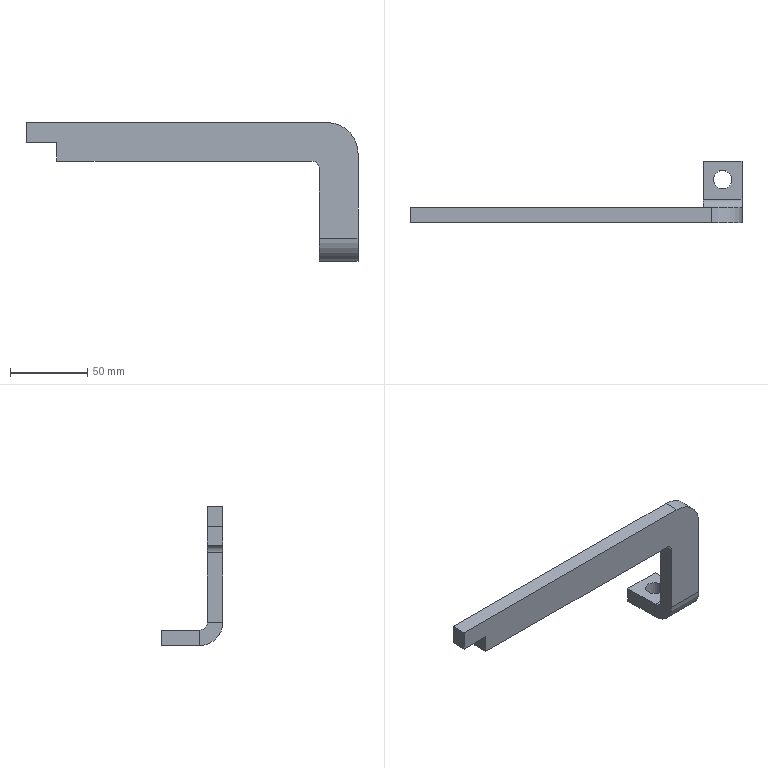Part | STEP file | Produce dryer HY-40-M-702 | 1 solid | 22 faces | box 215 x 40 x 90 mm | volume 72091 mm3 | plane 16 | cylinder 6 | commonest cylinder face diameters 10 x2 12 x2 30 x1 40 x1
STEP:
#1=CARTESIAN_POINT('',(196.5,18.,-90.));
#2=VERTEX_POINT('',#1);
#3=CARTESIAN_POINT('',(208.5,18.,-90.));
#4=VERTEX_POINT('',#3);
#5=CARTESIAN_POINT('',(202.5,18.,-90.));
#6=DIRECTION('',(0.,0.,1.));
#7=DIRECTION('',(1.,0.,0.));
#8=AXIS2_PLACEMENT_3D('',#5,#6,#7);
#9=CIRCLE('',#8,6.);
#10=EDGE_CURVE('',#2,#4,#9,.T.);
#11=ORIENTED_EDGE('',*,*,#10,.F.);
#12=CARTESIAN_POINT('',(196.5,18.,-80.));
#13=VERTEX_POINT('',#12);
#14=CARTESIAN_POINT('',(196.5,18.,-90.));
#15=DIRECTION('',(0.,0.,1.));
#16=VECTOR('',#15,1000.);
#17=LINE('',#14,#16);
#18=EDGE_CURVE('',#2,#13,#17,.T.);
#19=ORIENTED_EDGE('',*,*,#18,.T.);
#20=CARTESIAN_POINT('',(208.5,18.,-80.));
#21=VERTEX_POINT('',#20);
#22=CARTESIAN_POINT('',(202.5,18.,-80.));
#23=DIRECTION('',(0.,0.,1.));
#24=DIRECTION('',(1.,0.,0.));
#25=AXIS2_PLACEMENT_3D('',#22,#23,#24);
#26=CIRCLE('',#25,6.);
#27=EDGE_CURVE('',#13,#21,#26,.T.);
#28=ORIENTED_EDGE('',*,*,#27,.T.);
#29=CARTESIAN_POINT('',(208.5,18.,-90.));
#30=DIRECTION('',(0.,0.,1.));
#31=VECTOR('',#30,1000.);
#32=LINE('',#29,#31);
#33=EDGE_CURVE('',#4,#21,#32,.T.);
#34=ORIENTED_EDGE('',*,*,#33,.F.);
#35=EDGE_LOOP('',(#11,#19,#28,#34));
#36=FACE_OUTER_BOUND('',#35,.T.);
#37=CARTESIAN_POINT('',(202.5,18.,-90.));
#38=DIRECTION('',(0.,0.,1.));
#39=DIRECTION('',(1.,0.,0.));
#40=AXIS2_PLACEMENT_3D('',#37,#38,#39);
#41=CYLINDRICAL_SURFACE('',#40,6.);
#42=ADVANCED_FACE('',(#36),#41,.F.);
#43=CARTESIAN_POINT('',(190.,0.,-75.));
#44=VERTEX_POINT('',#43);
#45=CARTESIAN_POINT('',(190.,0.,-30.));
#46=VERTEX_POINT('',#45);
#47=CARTESIAN_POINT('',(190.,0.,-90.));
#48=DIRECTION('',(0.,0.,1.));
#49=VECTOR('',#48,1000.);
#50=LINE('',#47,#49);
#51=EDGE_CURVE('',#44,#46,#50,.T.);
#52=ORIENTED_EDGE('',*,*,#51,.F.);
#53=CARTESIAN_POINT('',(190.,-10.,-75.));
#54=VERTEX_POINT('',#53);
#55=CARTESIAN_POINT('',(190.,0.,-75.));
#56=DIRECTION('',(0.,-1.,0.));
#57=VECTOR('',#56,1000.);
#58=LINE('',#55,#57);
#59=EDGE_CURVE('',#44,#54,#58,.T.);
#60=ORIENTED_EDGE('',*,*,#59,.T.);
#61=CARTESIAN_POINT('',(190.,-10.,-30.));
#62=VERTEX_POINT('',#61);
#63=CARTESIAN_POINT('',(190.,-10.,-90.));
#64=DIRECTION('',(0.,0.,1.));
#65=VECTOR('',#64,1000.);
#66=LINE('',#63,#65);
#67=EDGE_CURVE('',#54,#62,#66,.T.);
#68=ORIENTED_EDGE('',*,*,#67,.T.);
#69=CARTESIAN_POINT('',(190.,-10.,-30.));
#70=DIRECTION('',(0.,1.,0.));
#71=VECTOR('',#70,1000.);
#72=LINE('',#69,#71);
#73=EDGE_CURVE('',#62,#46,#72,.T.);
#74=ORIENTED_EDGE('',*,*,#73,.T.);
#75=EDGE_LOOP('',(#52,#60,#68,#74));
#76=FACE_OUTER_BOUND('',#75,.T.);
#77=CARTESIAN_POINT('',(190.,-10.,-90.));
#78=DIRECTION('',(-1.,0.,0.));
#79=DIRECTION('',(0.,0.,1.));
#80=AXIS2_PLACEMENT_3D('',#77,#78,#79);
#81=PLANE('',#80);
#82=ADVANCED_FACE('',(#76),#81,.T.);
#83=CARTESIAN_POINT('',(215.,-10.,-75.));
#84=VERTEX_POINT('',#83);
#85=CARTESIAN_POINT('',(190.,-10.,-75.));
#86=DIRECTION('',(1.,0.,0.));
#87=VECTOR('',#86,1000.);
#88=LINE('',#85,#87);
#89=EDGE_CURVE('',#54,#84,#88,.T.);
#90=ORIENTED_EDGE('',*,*,#89,.T.);
#91=CARTESIAN_POINT('',(215.,-10.,-20.));
#92=VERTEX_POINT('',#91);
#93=CARTESIAN_POINT('',(215.,-10.,-20.));
#94=DIRECTION('',(0.,0.,-1.));
#95=VECTOR('',#94,1000.);
#96=LINE('',#93,#95);
#97=EDGE_CURVE('',#92,#84,#96,.T.);
#98=ORIENTED_EDGE('',*,*,#97,.F.);
#99=CARTESIAN_POINT('',(195.,-10.,0.));
#100=VERTEX_POINT('',#99);
#101=CARTESIAN_POINT('',(195.,-10.,-20.));
#102=DIRECTION('',(0.,1.,0.));
#103=DIRECTION('',(0.,0.,1.));
#104=AXIS2_PLACEMENT_3D('',#101,#102,#103);
#105=CIRCLE('',#104,20.);
#106=EDGE_CURVE('',#100,#92,#105,.T.);
#107=ORIENTED_EDGE('',*,*,#106,.F.);
#108=CARTESIAN_POINT('',(0.,-10.,0.));
#109=VERTEX_POINT('',#108);
#110=CARTESIAN_POINT('',(0.,-10.,0.));
#111=DIRECTION('',(1.,0.,0.));
#112=VECTOR('',#111,1000.);
#113=LINE('',#110,#112);
#114=EDGE_CURVE('',#109,#100,#113,.T.);
#115=ORIENTED_EDGE('',*,*,#114,.F.);
#116=CARTESIAN_POINT('',(0.,-10.,-13.));
#117=VERTEX_POINT('',#116);
#118=CARTESIAN_POINT('',(0.,-10.,-13.));
#119=DIRECTION('',(0.,0.,1.));
#120=VECTOR('',#119,1000.);
#121=LINE('',#118,#120);
#122=EDGE_CURVE('',#117,#109,#121,.T.);
#123=ORIENTED_EDGE('',*,*,#122,.F.);
#124=CARTESIAN_POINT('',(20.,-10.,-13.));
#125=VERTEX_POINT('',#124);
#126=CARTESIAN_POINT('',(0.,-10.,-13.));
#127=DIRECTION('',(-1.,0.,0.));
#128=VECTOR('',#127,1000.);
#129=LINE('',#126,#128);
#130=EDGE_CURVE('',#125,#117,#129,.T.);
#131=ORIENTED_EDGE('',*,*,#130,.F.);
#132=CARTESIAN_POINT('',(20.,-10.,-25.));
#133=VERTEX_POINT('',#132);
#134=CARTESIAN_POINT('',(20.,-10.,-25.));
#135=DIRECTION('',(0.,0.,1.));
#136=VECTOR('',#135,1000.);
#137=LINE('',#134,#136);
#138=EDGE_CURVE('',#133,#125,#137,.T.);
#139=ORIENTED_EDGE('',*,*,#138,.F.);
#140=CARTESIAN_POINT('',(185.,-10.,-25.));
#141=VERTEX_POINT('',#140);
#142=CARTESIAN_POINT('',(185.,-10.,-25.));
#143=DIRECTION('',(-1.,0.,0.));
#144=VECTOR('',#143,1000.);
#145=LINE('',#142,#144);
#146=EDGE_CURVE('',#141,#133,#145,.T.);
#147=ORIENTED_EDGE('',*,*,#146,.F.);
#148=CARTESIAN_POINT('',(185.,-10.,-30.));
#149=DIRECTION('',(0.,-1.,0.));
#150=DIRECTION('',(0.,0.,-1.));
#151=AXIS2_PLACEMENT_3D('',#148,#149,#150);
#152=CIRCLE('',#151,5.);
#153=EDGE_CURVE('',#62,#141,#152,.T.);
#154=ORIENTED_EDGE('',*,*,#153,.F.);
#155=ORIENTED_EDGE('',*,*,#67,.F.);
#156=EDGE_LOOP('',(#90,#98,#107,#115,#123,#131,#139,#147,#154,#155));
#157=FACE_OUTER_BOUND('',#156,.T.);
#158=CARTESIAN_POINT('',(195.,-10.,-20.));
#159=DIRECTION('',(0.,1.,0.));
#160=DIRECTION('',(0.,0.,1.));
#161=AXIS2_PLACEMENT_3D('',#158,#159,#160);
#162=PLANE('',#161);
#163=ADVANCED_FACE('',(#157),#162,.F.);
#164=CARTESIAN_POINT('',(215.,0.,-20.));
#165=VERTEX_POINT('',#164);
#166=CARTESIAN_POINT('',(215.,0.,-75.));
#167=VERTEX_POINT('',#166);
#168=CARTESIAN_POINT('',(215.,0.,-20.));
#169=DIRECTION('',(0.,0.,-1.));
#170=VECTOR('',#169,1000.);
#171=LINE('',#168,#170);
#172=EDGE_CURVE('',#165,#167,#171,.T.);
#173=ORIENTED_EDGE('',*,*,#172,.T.);
#174=CARTESIAN_POINT('',(190.,0.,-75.));
#175=DIRECTION('',(1.,0.,0.));
#176=VECTOR('',#175,1000.);
#177=LINE('',#174,#176);
#178=EDGE_CURVE('',#44,#167,#177,.T.);
#179=ORIENTED_EDGE('',*,*,#178,.F.);
#180=ORIENTED_EDGE('',*,*,#51,.T.);
#181=CARTESIAN_POINT('',(185.,0.,-25.));
#182=VERTEX_POINT('',#181);
#183=CARTESIAN_POINT('',(185.,0.,-30.));
#184=DIRECTION('',(0.,-1.,0.));
#185=DIRECTION('',(0.,0.,-1.));
#186=AXIS2_PLACEMENT_3D('',#183,#184,#185);
#187=CIRCLE('',#186,5.);
#188=EDGE_CURVE('',#46,#182,#187,.T.);
#189=ORIENTED_EDGE('',*,*,#188,.T.);
#190=CARTESIAN_POINT('',(20.,0.,-25.));
#191=VERTEX_POINT('',#190);
#192=CARTESIAN_POINT('',(185.,0.,-25.));
#193=DIRECTION('',(-1.,0.,0.));
#194=VECTOR('',#193,1000.);
#195=LINE('',#192,#194);
#196=EDGE_CURVE('',#182,#191,#195,.T.);
#197=ORIENTED_EDGE('',*,*,#196,.T.);
#198=CARTESIAN_POINT('',(20.,0.,-13.));
#199=VERTEX_POINT('',#198);
#200=CARTESIAN_POINT('',(20.,0.,-25.));
#201=DIRECTION('',(0.,0.,1.));
#202=VECTOR('',#201,1000.);
#203=LINE('',#200,#202);
#204=EDGE_CURVE('',#191,#199,#203,.T.);
#205=ORIENTED_EDGE('',*,*,#204,.T.);
#206=CARTESIAN_POINT('',(0.,0.,-13.));
#207=VERTEX_POINT('',#206);
#208=CARTESIAN_POINT('',(0.,0.,-13.));
#209=DIRECTION('',(-1.,0.,0.));
#210=VECTOR('',#209,1000.);
#211=LINE('',#208,#210);
#212=EDGE_CURVE('',#199,#207,#211,.T.);
#213=ORIENTED_EDGE('',*,*,#212,.T.);
#214=CARTESIAN_POINT('',(0.,0.,0.));
#215=VERTEX_POINT('',#214);
#216=CARTESIAN_POINT('',(0.,0.,-13.));
#217=DIRECTION('',(0.,0.,1.));
#218=VECTOR('',#217,1000.);
#219=LINE('',#216,#218);
#220=EDGE_CURVE('',#207,#215,#219,.T.);
#221=ORIENTED_EDGE('',*,*,#220,.T.);
#222=CARTESIAN_POINT('',(195.,0.,0.));
#223=VERTEX_POINT('',#222);
#224=CARTESIAN_POINT('',(0.,0.,0.));
#225=DIRECTION('',(1.,0.,0.));
#226=VECTOR('',#225,1000.);
#227=LINE('',#224,#226);
#228=EDGE_CURVE('',#215,#223,#227,.T.);
#229=ORIENTED_EDGE('',*,*,#228,.T.);
#230=CARTESIAN_POINT('',(195.,0.,-20.));
#231=DIRECTION('',(0.,1.,0.));
#232=DIRECTION('',(0.,0.,1.));
#233=AXIS2_PLACEMENT_3D('',#230,#231,#232);
#234=CIRCLE('',#233,20.);
#235=EDGE_CURVE('',#223,#165,#234,.T.);
#236=ORIENTED_EDGE('',*,*,#235,.T.);
#237=EDGE_LOOP('',(#173,#179,#180,#189,#197,#205,#213,#221,#229,#236));
#238=FACE_OUTER_BOUND('',#237,.T.);
#239=CARTESIAN_POINT('',(195.,0.,-20.));
#240=DIRECTION('',(0.,1.,0.));
#241=DIRECTION('',(0.,0.,1.));
#242=AXIS2_PLACEMENT_3D('',#239,#240,#241);
#243=PLANE('',#242);
#244=ADVANCED_FACE('',(#238),#243,.T.);
#245=ORIENTED_EDGE('',*,*,#220,.F.);
#246=CARTESIAN_POINT('',(0.,-10.,-13.));
#247=DIRECTION('',(0.,1.,0.));
#248=VECTOR('',#247,1000.);
#249=LINE('',#246,#248);
#250=EDGE_CURVE('',#117,#207,#249,.T.);
#251=ORIENTED_EDGE('',*,*,#250,.F.);
#252=ORIENTED_EDGE('',*,*,#122,.T.);
#253=CARTESIAN_POINT('',(0.,-10.,0.));
#254=DIRECTION('',(0.,1.,0.));
#255=VECTOR('',#254,1000.);
#256=LINE('',#253,#255);
#257=EDGE_CURVE('',#109,#215,#256,.T.);
#258=ORIENTED_EDGE('',*,*,#257,.T.);
#259=EDGE_LOOP('',(#245,#251,#252,#258));
#260=FACE_OUTER_BOUND('',#259,.T.);
#261=CARTESIAN_POINT('',(0.,-10.,-13.));
#262=DIRECTION('',(-1.,0.,0.));
#263=DIRECTION('',(0.,0.,1.));
#264=AXIS2_PLACEMENT_3D('',#261,#262,#263);
#265=PLANE('',#264);
#266=ADVANCED_FACE('',(#260),#265,.T.);
#267=ORIENTED_EDGE('',*,*,#212,.F.);
#268=CARTESIAN_POINT('',(20.,-10.,-13.));
#269=DIRECTION('',(0.,1.,0.));
#270=VECTOR('',#269,1000.);
#271=LINE('',#268,#270);
#272=EDGE_CURVE('',#125,#199,#271,.T.);
#273=ORIENTED_EDGE('',*,*,#272,.F.);
#274=ORIENTED_EDGE('',*,*,#130,.T.);
#275=ORIENTED_EDGE('',*,*,#250,.T.);
#276=EDGE_LOOP('',(#267,#273,#274,#275));
#277=FACE_OUTER_BOUND('',#276,.T.);
#278=CARTESIAN_POINT('',(0.,-10.,-13.));
#279=DIRECTION('',(0.,0.,-1.));
#280=DIRECTION('',(-1.,0.,0.));
#281=AXIS2_PLACEMENT_3D('',#278,#279,#280);
#282=PLANE('',#281);
#283=ADVANCED_FACE('',(#277),#282,.T.);
#284=ORIENTED_EDGE('',*,*,#204,.F.);
#285=CARTESIAN_POINT('',(20.,-10.,-25.));
#286=DIRECTION('',(0.,1.,0.));
#287=VECTOR('',#286,1000.);
#288=LINE('',#285,#287);
#289=EDGE_CURVE('',#133,#191,#288,.T.);
#290=ORIENTED_EDGE('',*,*,#289,.F.);
#291=ORIENTED_EDGE('',*,*,#138,.T.);
#292=ORIENTED_EDGE('',*,*,#272,.T.);
#293=EDGE_LOOP('',(#284,#290,#291,#292));
#294=FACE_OUTER_BOUND('',#293,.T.);
#295=CARTESIAN_POINT('',(20.,-10.,-25.));
#296=DIRECTION('',(-1.,0.,0.));
#297=DIRECTION('',(0.,0.,1.));
#298=AXIS2_PLACEMENT_3D('',#295,#296,#297);
#299=PLANE('',#298);
#300=ADVANCED_FACE('',(#294),#299,.T.);
#301=ORIENTED_EDGE('',*,*,#196,.F.);
#302=CARTESIAN_POINT('',(185.,-10.,-25.));
#303=DIRECTION('',(0.,1.,0.));
#304=VECTOR('',#303,1000.);
#305=LINE('',#302,#304);
#306=EDGE_CURVE('',#141,#182,#305,.T.);
#307=ORIENTED_EDGE('',*,*,#306,.F.);
#308=ORIENTED_EDGE('',*,*,#146,.T.);
#309=ORIENTED_EDGE('',*,*,#289,.T.);
#310=EDGE_LOOP('',(#301,#307,#308,#309));
#311=FACE_OUTER_BOUND('',#310,.T.);
#312=CARTESIAN_POINT('',(185.,-10.,-25.));
#313=DIRECTION('',(0.,0.,-1.));
#314=DIRECTION('',(-1.,0.,0.));
#315=AXIS2_PLACEMENT_3D('',#312,#313,#314);
#316=PLANE('',#315);
#317=ADVANCED_FACE('',(#311),#316,.T.);
#318=ORIENTED_EDGE('',*,*,#188,.F.);
#319=ORIENTED_EDGE('',*,*,#73,.F.);
#320=ORIENTED_EDGE('',*,*,#153,.T.);
#321=ORIENTED_EDGE('',*,*,#306,.T.);
#322=EDGE_LOOP('',(#318,#319,#320,#321));
#323=FACE_OUTER_BOUND('',#322,.T.);
#324=CARTESIAN_POINT('',(185.,-10.,-30.));
#325=DIRECTION('',(0.,1.,0.));
#326=DIRECTION('',(0.,0.,1.));
#327=AXIS2_PLACEMENT_3D('',#324,#325,#326);
#328=CYLINDRICAL_SURFACE('',#327,5.);
#329=ADVANCED_FACE('',(#323),#328,.F.);
#330=CARTESIAN_POINT('',(215.,0.,-75.));
#331=DIRECTION('',(0.,-1.,0.));
#332=VECTOR('',#331,1000.);
#333=LINE('',#330,#332);
#334=EDGE_CURVE('',#167,#84,#333,.T.);
#335=ORIENTED_EDGE('',*,*,#334,.F.);
#336=ORIENTED_EDGE('',*,*,#172,.F.);
#337=CARTESIAN_POINT('',(215.,-10.,-20.));
#338=DIRECTION('',(0.,1.,0.));
#339=VECTOR('',#338,1000.);
#340=LINE('',#337,#339);
#341=EDGE_CURVE('',#92,#165,#340,.T.);
#342=ORIENTED_EDGE('',*,*,#341,.F.);
#343=ORIENTED_EDGE('',*,*,#97,.T.);
#344=EDGE_LOOP('',(#335,#336,#342,#343));
#345=FACE_OUTER_BOUND('',#344,.T.);
#346=CARTESIAN_POINT('',(215.,-10.,-20.));
#347=DIRECTION('',(1.,0.,0.));
#348=DIRECTION('',(0.,0.,-1.));
#349=AXIS2_PLACEMENT_3D('',#346,#347,#348);
#350=PLANE('',#349);
#351=ADVANCED_FACE('',(#345),#350,.T.);
#352=ORIENTED_EDGE('',*,*,#235,.F.);
#353=CARTESIAN_POINT('',(195.,-10.,0.));
#354=DIRECTION('',(0.,1.,0.));
#355=VECTOR('',#354,1000.);
#356=LINE('',#353,#355);
#357=EDGE_CURVE('',#100,#223,#356,.T.);
#358=ORIENTED_EDGE('',*,*,#357,.F.);
#359=ORIENTED_EDGE('',*,*,#106,.T.);
#360=ORIENTED_EDGE('',*,*,#341,.T.);
#361=EDGE_LOOP('',(#352,#358,#359,#360));
#362=FACE_OUTER_BOUND('',#361,.T.);
#363=CARTESIAN_POINT('',(195.,-10.,-20.));
#364=DIRECTION('',(0.,1.,0.));
#365=DIRECTION('',(0.,0.,1.));
#366=AXIS2_PLACEMENT_3D('',#363,#364,#365);
#367=CYLINDRICAL_SURFACE('',#366,20.);
#368=ADVANCED_FACE('',(#362),#367,.T.);
#369=ORIENTED_EDGE('',*,*,#228,.F.);
#370=ORIENTED_EDGE('',*,*,#257,.F.);
#371=ORIENTED_EDGE('',*,*,#114,.T.);
#372=ORIENTED_EDGE('',*,*,#357,.T.);
#373=EDGE_LOOP('',(#369,#370,#371,#372));
#374=FACE_OUTER_BOUND('',#373,.T.);
#375=CARTESIAN_POINT('',(0.,-10.,0.));
#376=DIRECTION('',(0.,0.,1.));
#377=DIRECTION('',(1.,0.,0.));
#378=AXIS2_PLACEMENT_3D('',#375,#376,#377);
#379=PLANE('',#378);
#380=ADVANCED_FACE('',(#374),#379,.T.);
#381=CARTESIAN_POINT('',(215.,5.,-80.));
#382=VERTEX_POINT('',#381);
#383=CARTESIAN_POINT('',(215.,5.,-90.));
#384=VERTEX_POINT('',#383);
#385=CARTESIAN_POINT('',(215.,5.,-90.));
#386=DIRECTION('',(0.,0.,-1.));
#387=VECTOR('',#386,1000.);
#388=LINE('',#385,#387);
#389=EDGE_CURVE('',#382,#384,#388,.T.);
#390=ORIENTED_EDGE('',*,*,#389,.F.);
#391=CARTESIAN_POINT('',(215.,5.,-75.));
#392=DIRECTION('',(1.,0.,0.));
#393=DIRECTION('',(0.,0.,1.));
#394=AXIS2_PLACEMENT_3D('',#391,#392,#393);
#395=CIRCLE('',#394,5.);
#396=EDGE_CURVE('',#167,#382,#395,.T.);
#397=ORIENTED_EDGE('',*,*,#396,.F.);
#398=ORIENTED_EDGE('',*,*,#334,.T.);
#399=CARTESIAN_POINT('',(215.,5.,-75.));
#400=DIRECTION('',(1.,0.,0.));
#401=DIRECTION('',(0.,0.,1.));
#402=AXIS2_PLACEMENT_3D('',#399,#400,#401);
#403=CIRCLE('',#402,15.);
#404=EDGE_CURVE('',#84,#384,#403,.T.);
#405=ORIENTED_EDGE('',*,*,#404,.T.);
#406=EDGE_LOOP('',(#390,#397,#398,#405));
#407=FACE_OUTER_BOUND('',#406,.T.);
#408=CARTESIAN_POINT('',(215.,5.,-75.));
#409=DIRECTION('',(1.,0.,0.));
#410=DIRECTION('',(0.,0.,-1.));
#411=AXIS2_PLACEMENT_3D('',#408,#409,#410);
#412=PLANE('',#411);
#413=ADVANCED_FACE('',(#407),#412,.T.);
#414=CARTESIAN_POINT('',(190.,5.,-80.));
#415=VERTEX_POINT('',#414);
#416=CARTESIAN_POINT('',(190.,5.,-75.));
#417=DIRECTION('',(-1.,0.,0.));
#418=DIRECTION('',(0.,0.,1.));
#419=AXIS2_PLACEMENT_3D('',#416,#417,#418);
#420=CIRCLE('',#419,5.);
#421=EDGE_CURVE('',#415,#44,#420,.T.);
#422=ORIENTED_EDGE('',*,*,#421,.F.);
#423=CARTESIAN_POINT('',(190.,5.,-90.));
#424=VERTEX_POINT('',#423);
#425=CARTESIAN_POINT('',(190.,5.,-80.));
#426=DIRECTION('',(0.,0.,-1.));
#427=VECTOR('',#426,1000.);
#428=LINE('',#425,#427);
#429=EDGE_CURVE('',#415,#424,#428,.T.);
#430=ORIENTED_EDGE('',*,*,#429,.T.);
#431=CARTESIAN_POINT('',(190.,5.,-75.));
#432=DIRECTION('',(-1.,0.,0.));
#433=DIRECTION('',(0.,0.,1.));
#434=AXIS2_PLACEMENT_3D('',#431,#432,#433);
#435=CIRCLE('',#434,15.);
#436=EDGE_CURVE('',#424,#54,#435,.T.);
#437=ORIENTED_EDGE('',*,*,#436,.T.);
#438=ORIENTED_EDGE('',*,*,#59,.F.);
#439=EDGE_LOOP('',(#422,#430,#437,#438));
#440=FACE_OUTER_BOUND('',#439,.T.);
#441=CARTESIAN_POINT('',(190.,5.,-75.));
#442=DIRECTION('',(1.,0.,0.));
#443=DIRECTION('',(0.,0.,-1.));
#444=AXIS2_PLACEMENT_3D('',#441,#442,#443);
#445=PLANE('',#444);
#446=ADVANCED_FACE('',(#440),#445,.F.);
#447=ORIENTED_EDGE('',*,*,#89,.F.);
#448=ORIENTED_EDGE('',*,*,#436,.F.);
#449=CARTESIAN_POINT('',(0.,5.,-90.));
#450=DIRECTION('',(-1.,0.,0.));
#451=VECTOR('',#450,1000.);
#452=LINE('',#449,#451);
#453=EDGE_CURVE('',#384,#424,#452,.T.);
#454=ORIENTED_EDGE('',*,*,#453,.F.);
#455=ORIENTED_EDGE('',*,*,#404,.F.);
#456=EDGE_LOOP('',(#447,#448,#454,#455));
#457=FACE_OUTER_BOUND('',#456,.T.);
#458=CARTESIAN_POINT('',(190.,5.,-75.));
#459=DIRECTION('',(-1.,0.,0.));
#460=DIRECTION('',(0.,0.,-1.));
#461=AXIS2_PLACEMENT_3D('',#458,#459,#460);
#462=CYLINDRICAL_SURFACE('',#461,15.);
#463=ADVANCED_FACE('',(#457),#462,.T.);
#464=ORIENTED_EDGE('',*,*,#178,.T.);
#465=ORIENTED_EDGE('',*,*,#396,.T.);
#466=CARTESIAN_POINT('',(215.,5.,-80.));
#467=DIRECTION('',(-1.,0.,0.));
#468=VECTOR('',#467,1000.);
#469=LINE('',#466,#468);
#470=EDGE_CURVE('',#382,#415,#469,.T.);
#471=ORIENTED_EDGE('',*,*,#470,.T.);
#472=ORIENTED_EDGE('',*,*,#421,.T.);
#473=EDGE_LOOP('',(#464,#465,#471,#472));
#474=FACE_OUTER_BOUND('',#473,.T.);
#475=CARTESIAN_POINT('',(190.,5.,-75.));
#476=DIRECTION('',(-1.,0.,0.));
#477=DIRECTION('',(0.,0.,-1.));
#478=AXIS2_PLACEMENT_3D('',#475,#476,#477);
#479=CYLINDRICAL_SURFACE('',#478,5.);
#480=ADVANCED_FACE('',(#474),#479,.F.);
#481=CARTESIAN_POINT('',(190.,30.,-90.));
#482=VERTEX_POINT('',#481);
#483=CARTESIAN_POINT('',(190.,0.,-90.));
#484=DIRECTION('',(0.,-1.,0.));
#485=VECTOR('',#484,1000.);
#486=LINE('',#483,#485);
#487=EDGE_CURVE('',#482,#424,#486,.T.);
#488=ORIENTED_EDGE('',*,*,#487,.T.);
#489=ORIENTED_EDGE('',*,*,#429,.F.);
#490=CARTESIAN_POINT('',(190.,30.,-80.));
#491=VERTEX_POINT('',#490);
#492=CARTESIAN_POINT('',(190.,0.,-80.));
#493=DIRECTION('',(0.,-1.,0.));
#494=VECTOR('',#493,1000.);
#495=LINE('',#492,#494);
#496=EDGE_CURVE('',#491,#415,#495,.T.);
#497=ORIENTED_EDGE('',*,*,#496,.F.);
#498=CARTESIAN_POINT('',(190.,30.,-90.));
#499=DIRECTION('',(0.,0.,1.));
#500=VECTOR('',#499,1000.);
#501=LINE('',#498,#500);
#502=EDGE_CURVE('',#482,#491,#501,.T.);
#503=ORIENTED_EDGE('',*,*,#502,.F.);
#504=EDGE_LOOP('',(#488,#489,#497,#503));
#505=FACE_OUTER_BOUND('',#504,.T.);
#506=CARTESIAN_POINT('',(190.,0.,-90.));
#507=DIRECTION('',(-1.,0.,0.));
#508=DIRECTION('',(0.,0.,1.));
#509=AXIS2_PLACEMENT_3D('',#506,#507,#508);
#510=PLANE('',#509);
#511=ADVANCED_FACE('',(#505),#510,.T.);
#512=CARTESIAN_POINT('',(215.,30.,-80.));
#513=VERTEX_POINT('',#512);
#514=CARTESIAN_POINT('',(215.,0.,-80.));
#515=DIRECTION('',(0.,1.,0.));
#516=VECTOR('',#515,1000.);
#517=LINE('',#514,#516);
#518=EDGE_CURVE('',#382,#513,#517,.T.);
#519=ORIENTED_EDGE('',*,*,#518,.F.);
#520=ORIENTED_EDGE('',*,*,#389,.T.);
#521=CARTESIAN_POINT('',(215.,30.,-90.));
#522=VERTEX_POINT('',#521);
#523=CARTESIAN_POINT('',(215.,30.,-90.));
#524=DIRECTION('',(0.,1.,0.));
#525=VECTOR('',#524,1000.);
#526=LINE('',#523,#525);
#527=EDGE_CURVE('',#384,#522,#526,.T.);
#528=ORIENTED_EDGE('',*,*,#527,.T.);
#529=CARTESIAN_POINT('',(215.,30.,-90.));
#530=DIRECTION('',(0.,0.,1.));
#531=VECTOR('',#530,1000.);
#532=LINE('',#529,#531);
#533=EDGE_CURVE('',#522,#513,#532,.T.);
#534=ORIENTED_EDGE('',*,*,#533,.T.);
#535=EDGE_LOOP('',(#519,#520,#528,#534));
#536=FACE_OUTER_BOUND('',#535,.T.);
#537=CARTESIAN_POINT('',(215.,30.,-90.));
#538=DIRECTION('',(1.,0.,0.));
#539=DIRECTION('',(0.,0.,-1.));
#540=AXIS2_PLACEMENT_3D('',#537,#538,#539);
#541=PLANE('',#540);
#542=ADVANCED_FACE('',(#536),#541,.T.);
#543=CARTESIAN_POINT('',(202.5,18.,-90.));
#544=DIRECTION('',(0.,0.,1.));
#545=DIRECTION('',(1.,0.,0.));
#546=AXIS2_PLACEMENT_3D('',#543,#544,#545);
#547=CIRCLE('',#546,6.);
#548=EDGE_CURVE('',#4,#2,#547,.T.);
#549=ORIENTED_EDGE('',*,*,#548,.T.);
#550=ORIENTED_EDGE('',*,*,#10,.T.);
#551=EDGE_LOOP('',(#549,#550));
#552=FACE_BOUND('',#551,.T.);
#553=ORIENTED_EDGE('',*,*,#527,.F.);
#554=ORIENTED_EDGE('',*,*,#453,.T.);
#555=ORIENTED_EDGE('',*,*,#487,.F.);
#556=CARTESIAN_POINT('',(190.,30.,-90.));
#557=DIRECTION('',(-1.,0.,0.));
#558=VECTOR('',#557,1000.);
#559=LINE('',#556,#558);
#560=EDGE_CURVE('',#522,#482,#559,.T.);
#561=ORIENTED_EDGE('',*,*,#560,.F.);
#562=EDGE_LOOP('',(#553,#554,#555,#561));
#563=FACE_OUTER_BOUND('',#562,.T.);
#564=CARTESIAN_POINT('',(0.,0.,-90.));
#565=DIRECTION('',(0.,0.,-1.));
#566=DIRECTION('',(-1.,0.,0.));
#567=AXIS2_PLACEMENT_3D('',#564,#565,#566);
#568=PLANE('',#567);
#569=ADVANCED_FACE('',(#552,#563),#568,.T.);
#570=CARTESIAN_POINT('',(202.5,18.,-80.));
#571=DIRECTION('',(0.,0.,1.));
#572=DIRECTION('',(1.,0.,0.));
#573=AXIS2_PLACEMENT_3D('',#570,#571,#572);
#574=CIRCLE('',#573,6.);
#575=EDGE_CURVE('',#21,#13,#574,.T.);
#576=ORIENTED_EDGE('',*,*,#575,.F.);
#577=ORIENTED_EDGE('',*,*,#27,.F.);
#578=EDGE_LOOP('',(#576,#577));
#579=FACE_BOUND('',#578,.T.);
#580=ORIENTED_EDGE('',*,*,#470,.F.);
#581=ORIENTED_EDGE('',*,*,#518,.T.);
#582=CARTESIAN_POINT('',(0.,30.,-80.));
#583=DIRECTION('',(-1.,0.,0.));
#584=VECTOR('',#583,1000.);
#585=LINE('',#582,#584);
#586=EDGE_CURVE('',#513,#491,#585,.T.);
#587=ORIENTED_EDGE('',*,*,#586,.T.);
#588=ORIENTED_EDGE('',*,*,#496,.T.);
#589=EDGE_LOOP('',(#580,#581,#587,#588));
#590=FACE_OUTER_BOUND('',#589,.T.);
#591=CARTESIAN_POINT('',(0.,0.,-80.));
#592=DIRECTION('',(0.,0.,-1.));
#593=DIRECTION('',(-1.,0.,0.));
#594=AXIS2_PLACEMENT_3D('',#591,#592,#593);
#595=PLANE('',#594);
#596=ADVANCED_FACE('',(#579,#590),#595,.F.);
#597=ORIENTED_EDGE('',*,*,#586,.F.);
#598=ORIENTED_EDGE('',*,*,#533,.F.);
#599=ORIENTED_EDGE('',*,*,#560,.T.);
#600=ORIENTED_EDGE('',*,*,#502,.T.);
#601=EDGE_LOOP('',(#597,#598,#599,#600));
#602=FACE_OUTER_BOUND('',#601,.T.);
#603=CARTESIAN_POINT('',(190.,30.,-90.));
#604=DIRECTION('',(0.,1.,0.));
#605=DIRECTION('',(0.,0.,1.));
#606=AXIS2_PLACEMENT_3D('',#603,#604,#605);
#607=PLANE('',#606);
#608=ADVANCED_FACE('',(#602),#607,.T.);
#609=ORIENTED_EDGE('',*,*,#18,.F.);
#610=ORIENTED_EDGE('',*,*,#548,.F.);
#611=ORIENTED_EDGE('',*,*,#33,.T.);
#612=ORIENTED_EDGE('',*,*,#575,.T.);
#613=EDGE_LOOP('',(#609,#610,#611,#612));
#614=FACE_OUTER_BOUND('',#613,.T.);
#615=CARTESIAN_POINT('',(202.5,18.,-90.));
#616=DIRECTION('',(0.,0.,1.));
#617=DIRECTION('',(1.,0.,0.));
#618=AXIS2_PLACEMENT_3D('',#615,#616,#617);
#619=CYLINDRICAL_SURFACE('',#618,6.);
#620=ADVANCED_FACE('',(#614),#619,.F.);
#621=CLOSED_SHELL('',(#42,#82,#163,#244,#266,#283,#300,#317,#329,#351,#368,#380,#413,#446,#463,#480,#511,#542,#569,#596,#608,#620));
#622=MANIFOLD_SOLID_BREP('',#621);
#623=CARTESIAN_POINT('',(0.,0.,0.));
#624=DIRECTION('',(0.,0.,1.));
#625=DIRECTION('',(1.,0.,0.));
#626=AXIS2_PLACEMENT_3D('',#623,#624,#625);
#627=(LENGTH_UNIT()NAMED_UNIT(*)SI_UNIT(.MILLI.,.METRE.));
#628=UNCERTAINTY_MEASURE_WITH_UNIT(LENGTH_MEASURE(0.00001),#627,'','');
#629=(NAMED_UNIT(*)PLANE_ANGLE_UNIT()SI_UNIT($,.RADIAN.));
#630=(NAMED_UNIT(*)SI_UNIT($,.STERADIAN.)SOLID_ANGLE_UNIT());
#631=(GEOMETRIC_REPRESENTATION_CONTEXT(3)GLOBAL_UNCERTAINTY_ASSIGNED_CONTEXT((#628))GLOBAL_UNIT_ASSIGNED_CONTEXT((#627,#629,#630))REPRESENTATION_CONTEXT('',''));
#632=ADVANCED_BREP_SHAPE_REPRESENTATION('',(#622,#626),#631);